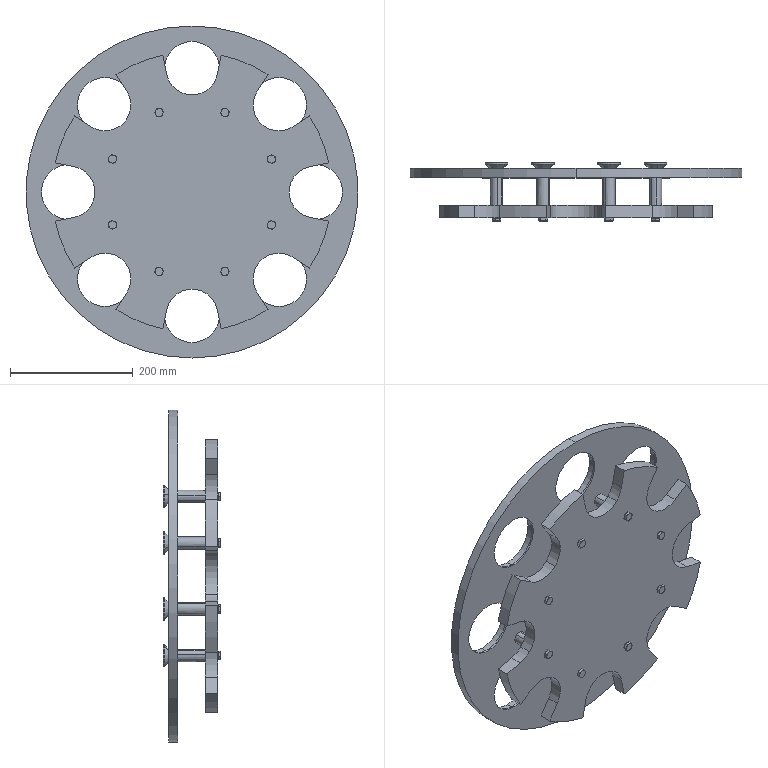Part | SolidWorks | 26 solids | 659 faces | box 540 x 94.26 x 540 mm | volume 5278659 mm3 | plane 252 | cylinder 207 | cone 184 | spline 16 | commonest cylinder face diameters 20 x64 8 x16 8.5 x16 11 x16 12 x16 36.05 x16